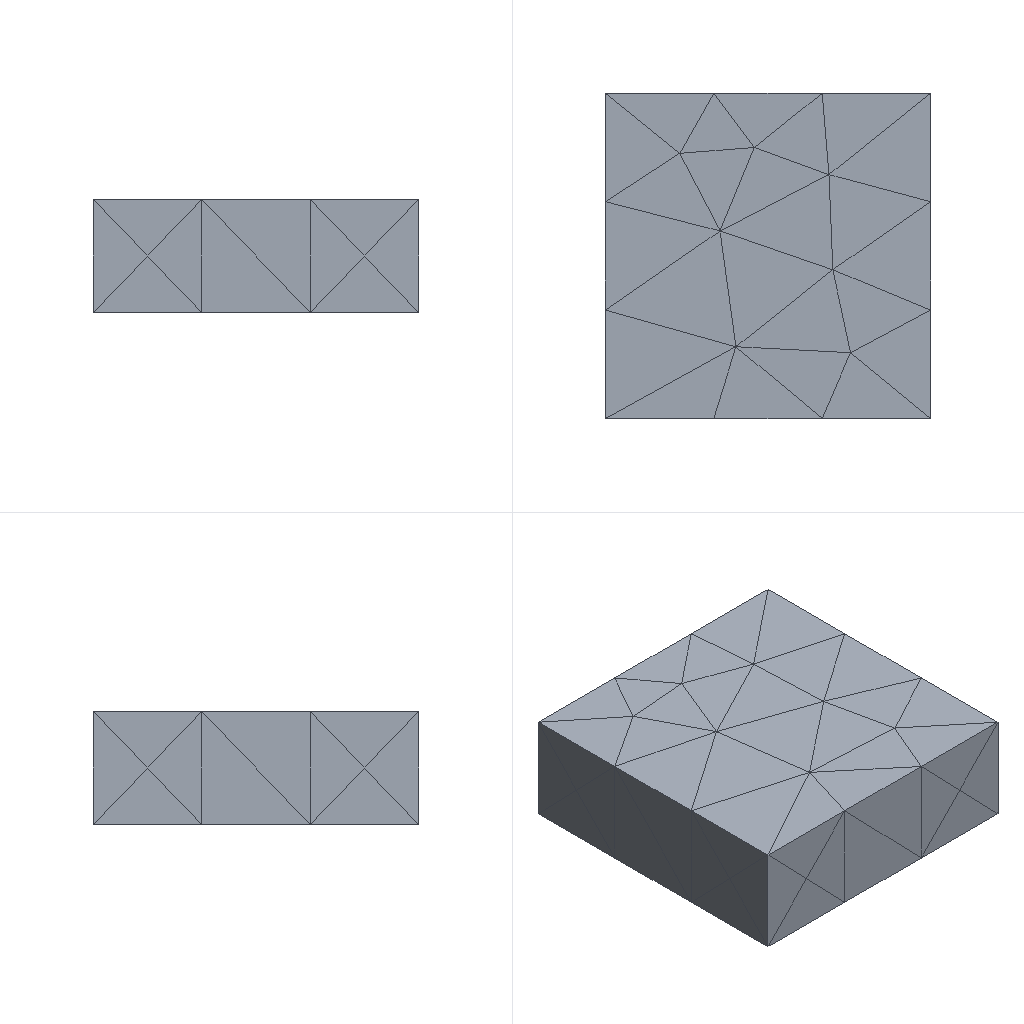Simulation study | ansys mapdl
Set-up summary:
category,name,step,type,value,unit,region
solver,ansys_mapdl
units,mm-N-s-tonne (MPa),,inferred,E=210000 density=
analysis,model,,static
mesh,nodes,,,240
mesh,elements,,,103
element_type,SOLID187,,,103
material,mat 1,,E,210000
material,mat 1,,nu,0.3
load,,model,body load temp,,,all
load,,model,force,"1000 [dir=(0, 0, -1) n=91]",,node list
bc,,model,fixed,"[dofs=UX,UY,UZ n=334]",,node list
Ansys APDL input file, long lists of numbers shortened:
/COM,ANSYS RELEASE 2026 R1           BUILD 26.1      UP20260202       09:08:10
/PREP7
/NOPR
/TITLE,2
ANTYPE, 0
*IF,_CDRDOFF,EQ,1,THEN     !if solid model was read in
_CDRDOFF=             !reset flag, numoffs already performed
*ELSE              !offset database for the following FE model
NUMOFF,NODE,      240
NUMOFF,ELEM,      103
NUMOFF,MAT ,        1
NUMOFF,TYPE,        1
*ENDIF
*SET,_RETURN ,  0.
*SET,_STATUS ,  0.
*SET,_UIQR   ,  91.
*SET,__FLOATPARAMETER__,  240.
DOF,DELETE
ETBLOCK,        1,        1
(2i9,19a9)
        1      187        0        0        0        0        0        0        0        0        0        0        0        0        0        0        0        0        0        0        0
       -1
NBLOCK,6,SOLID,       240,       240
(3i9,6e21.13e3)
        1        0        0 0.0000000000000E+000 2.9000000000000E+001 9.1000000000000E+001
! (239 more lines like these left out)
N,UNBL,LOC,       -1,
EBLOCK,19,SOLID,       103,       103
(19i10)
         1         1         1         1         0         0         0         0        10         0         1        84       164        60       119       157       180       181       107
! (205 more lines like these left out)
        -1
MPTEMP,UNBL, 1, 1,  0.    ,
MPDATA,UNBL, 1,EX  ,       1, 1,  210000.000    ,
MPTEMP,UNBL, 1, 1,  0.    ,
MPDATA,UNBL, 1,NUXY,       1, 1, 0.3    ,
MPTEMP,UNBL, 1, 1,  0.    ,
MPDATA,UNBL, 1,PRXY,       1, 1, 0.3    ,
EXTOPT,ATTR,      0,      0,      0
EXTOPT,ESIZE,  0,  0.
EXTOPT,ACLEAR,      0
TREF,  0.
IRLF,  0
BFUNIF,TEMP,_TINY
ACEL,  0.    ,  0.    ,  0.
OMEGA,  0.    ,  0.    ,  0.
DOMEGA,  0.    ,  0.    ,  0.
CGLOC,  0.    ,  0.    ,  0.
CGOMEGA,  0.    ,  0.    ,  0.
DCGOMG,  0.    ,  0.    ,  0.
KUSE,     0
TIME,  0.
ALPHAD,  0.
BETAD,  0.
DMPRAT,  0.
DMPSTR,  0.
CRPLIM, 0.1    ,   0
CRPLIM,  0.    ,   1
NCNV,     0, 1.000000000E+12,     0,  0.    ,  0.
NEQIT,     0
ERESX,DEFA
DBLOCK,       334
(i9,a6,2(pg16.9))
        1  UX    0.00000000      0.00000000
! (333 more lines like these left out)
       -1
FBLOCK,        91
(i9,a6,2(pg16.9))
       62  FZ   -10.9890110      0.00000000
! (90 more lines like these left out)
       -1
/GO
FINISH
Results summary:
result,analysis_type_db,,,static,unstated
result,n_sets,,,1,unstated
result,load_steps[0].set,load_step=1,,1,unstated
result,load_steps[0].substep,load_step=1,,1,unstated
result,load_steps[0].time,load_step=1,,1,unstated
result,load_steps[0].freq,load_step=1,,1,unstated
result,load_steps[0].max_usum,load_step=1,,0.000154,unstated
result,load_steps[0].max_seqv,load_step=1,,4.242,unstated
result,load_steps[0].reaction_sum.FX,load_step=1,,-6.35936e-13,unstated
result,load_steps[0].reaction_sum.FY,load_step=1,,-5.85487e-12,unstated
result,load_steps[0].reaction_sum.FZ,load_step=1,,1000,unstated
result,load_steps[0].reaction_sum.MX,load_step=1,,0,unstated
result,load_steps[0].reaction_sum.MY,load_step=1,,0,unstated
result,load_steps[0].reaction_sum.MZ,load_step=1,,0,unstated
result,convergence,,,results present for all listed sets,unstated